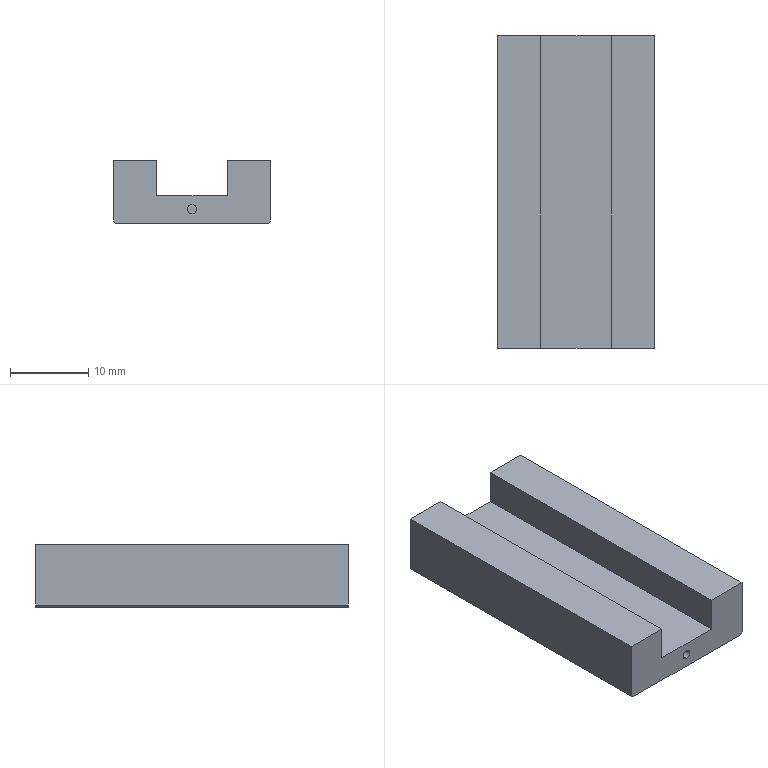Part | SolidWorks | features ICE 3, 3DProfileFeature 1, Chamfer 1, Extrusion 1, HoleWzd 1 | 1 solid | 31 faces | box 20 x 39.9 x 8 mm | volume 4656 mm3 | plane 13 | cylinder 10 | cone 8 | commonest cylinder face diameters 2.5 x8 1.2 x2
STEP:
#1=CARTESIAN_POINT('',(8.75,11.95,1.));
#2=VERTEX_POINT('',#1);
#3=CARTESIAN_POINT('',(6.25,11.95,1.));
#4=VERTEX_POINT('',#3);
#5=CARTESIAN_POINT('',(7.5,11.95,1.));
#6=DIRECTION('',(0.,0.,-1.));
#7=DIRECTION('',(-1.,0.,0.));
#8=AXIS2_PLACEMENT_3D('',#5,#6,#7);
#9=CIRCLE('',#8,1.25);
#10=EDGE_CURVE('',#2,#4,#9,.T.);
#11=ORIENTED_EDGE('',*,*,#10,.F.);
#12=CARTESIAN_POINT('',(8.75,11.95,-4.));
#13=VERTEX_POINT('',#12);
#14=CARTESIAN_POINT('',(8.75,11.95,-4.));
#15=DIRECTION('',(0.,0.,-1.));
#16=VECTOR('',#15,1000.);
#17=LINE('',#14,#16);
#18=EDGE_CURVE('',#2,#13,#17,.T.);
#19=ORIENTED_EDGE('',*,*,#18,.T.);
#20=CARTESIAN_POINT('',(6.25,11.95,-4.));
#21=VERTEX_POINT('',#20);
#22=CARTESIAN_POINT('',(7.5,11.95,-4.));
#23=DIRECTION('',(0.,0.,-1.));
#24=DIRECTION('',(-1.,0.,0.));
#25=AXIS2_PLACEMENT_3D('',#22,#23,#24);
#26=CIRCLE('',#25,1.25);
#27=EDGE_CURVE('',#13,#21,#26,.T.);
#28=ORIENTED_EDGE('',*,*,#27,.T.);
#29=CARTESIAN_POINT('',(6.25,11.95,-4.));
#30=DIRECTION('',(0.,0.,-1.));
#31=VECTOR('',#30,1000.);
#32=LINE('',#29,#31);
#33=EDGE_CURVE('',#4,#21,#32,.T.);
#34=ORIENTED_EDGE('',*,*,#33,.F.);
#35=EDGE_LOOP('',(#11,#19,#28,#34));
#36=FACE_OUTER_BOUND('',#35,.T.);
#37=CARTESIAN_POINT('',(7.5,11.95,-4.));
#38=DIRECTION('',(0.,0.,-1.));
#39=DIRECTION('',(-1.,0.,0.));
#40=AXIS2_PLACEMENT_3D('',#37,#38,#39);
#41=CYLINDRICAL_SURFACE('',#40,1.25);
#42=ADVANCED_FACE('',(#36),#41,.F.);
#43=CARTESIAN_POINT('',(7.5,11.95,1.751));
#44=VERTEX_POINT('',#43);
#45=CARTESIAN_POINT('',(6.25,11.95,1.));
#46=DIRECTION('',(-0.8572,0.,-0.515));
#47=VECTOR('',#46,1000.);
#48=LINE('',#45,#47);
#49=EDGE_CURVE('',#44,#4,#48,.T.);
#50=ORIENTED_EDGE('',*,*,#49,.F.);
#51=CARTESIAN_POINT('',(8.75,11.95,1.));
#52=DIRECTION('',(0.8572,0.,-0.515));
#53=VECTOR('',#52,1000.);
#54=LINE('',#51,#53);
#55=EDGE_CURVE('',#44,#2,#54,.T.);
#56=ORIENTED_EDGE('',*,*,#55,.T.);
#57=ORIENTED_EDGE('',*,*,#10,.T.);
#58=EDGE_LOOP('',(#50,#56,#57));
#59=FACE_OUTER_BOUND('',#58,.T.);
#60=CARTESIAN_POINT('',(7.5,11.95,1.));
#61=DIRECTION('',(0.,0.,-1.));
#62=DIRECTION('',(-1.,0.,0.));
#63=AXIS2_PLACEMENT_3D('',#60,#61,#62);
#64=CONICAL_SURFACE('',#63,1.25,1.03);
#65=ADVANCED_FACE('',(#59),#64,.F.);
#66=CARTESIAN_POINT('',(-6.25,11.95,1.));
#67=VERTEX_POINT('',#66);
#68=CARTESIAN_POINT('',(-8.75,11.95,1.));
#69=VERTEX_POINT('',#68);
#70=CARTESIAN_POINT('',(-7.5,11.95,1.));
#71=DIRECTION('',(0.,0.,-1.));
#72=DIRECTION('',(-1.,0.,0.));
#73=AXIS2_PLACEMENT_3D('',#70,#71,#72);
#74=CIRCLE('',#73,1.25);
#75=EDGE_CURVE('',#67,#69,#74,.T.);
#76=ORIENTED_EDGE('',*,*,#75,.F.);
#77=CARTESIAN_POINT('',(-6.25,11.95,-4.));
#78=VERTEX_POINT('',#77);
#79=CARTESIAN_POINT('',(-6.25,11.95,-4.));
#80=DIRECTION('',(0.,0.,-1.));
#81=VECTOR('',#80,1000.);
#82=LINE('',#79,#81);
#83=EDGE_CURVE('',#67,#78,#82,.T.);
#84=ORIENTED_EDGE('',*,*,#83,.T.);
#85=CARTESIAN_POINT('',(-8.75,11.95,-4.));
#86=VERTEX_POINT('',#85);
#87=CARTESIAN_POINT('',(-7.5,11.95,-4.));
#88=DIRECTION('',(0.,0.,-1.));
#89=DIRECTION('',(-1.,0.,0.));
#90=AXIS2_PLACEMENT_3D('',#87,#88,#89);
#91=CIRCLE('',#90,1.25);
#92=EDGE_CURVE('',#78,#86,#91,.T.);
#93=ORIENTED_EDGE('',*,*,#92,.T.);
#94=CARTESIAN_POINT('',(-8.75,11.95,-4.));
#95=DIRECTION('',(0.,0.,-1.));
#96=VECTOR('',#95,1000.);
#97=LINE('',#94,#96);
#98=EDGE_CURVE('',#69,#86,#97,.T.);
#99=ORIENTED_EDGE('',*,*,#98,.F.);
#100=EDGE_LOOP('',(#76,#84,#93,#99));
#101=FACE_OUTER_BOUND('',#100,.T.);
#102=CARTESIAN_POINT('',(-7.5,11.95,-4.));
#103=DIRECTION('',(0.,0.,-1.));
#104=DIRECTION('',(-1.,0.,0.));
#105=AXIS2_PLACEMENT_3D('',#102,#103,#104);
#106=CYLINDRICAL_SURFACE('',#105,1.25);
#107=ADVANCED_FACE('',(#101),#106,.F.);
#108=CARTESIAN_POINT('',(-7.5,11.95,1.751));
#109=VERTEX_POINT('',#108);
#110=CARTESIAN_POINT('',(-8.75,11.95,1.));
#111=DIRECTION('',(-0.8572,0.,-0.515));
#112=VECTOR('',#111,1000.);
#113=LINE('',#110,#112);
#114=EDGE_CURVE('',#109,#69,#113,.T.);
#115=ORIENTED_EDGE('',*,*,#114,.F.);
#116=CARTESIAN_POINT('',(-6.25,11.95,1.));
#117=DIRECTION('',(0.8572,0.,-0.515));
#118=VECTOR('',#117,1000.);
#119=LINE('',#116,#118);
#120=EDGE_CURVE('',#109,#67,#119,.T.);
#121=ORIENTED_EDGE('',*,*,#120,.T.);
#122=ORIENTED_EDGE('',*,*,#75,.T.);
#123=EDGE_LOOP('',(#115,#121,#122));
#124=FACE_OUTER_BOUND('',#123,.T.);
#125=CARTESIAN_POINT('',(-7.5,11.95,1.));
#126=DIRECTION('',(0.,0.,-1.));
#127=DIRECTION('',(-1.,0.,0.));
#128=AXIS2_PLACEMENT_3D('',#125,#126,#127);
#129=CONICAL_SURFACE('',#128,1.25,1.03);
#130=ADVANCED_FACE('',(#124),#129,.F.);
#131=CARTESIAN_POINT('',(-6.25,27.95,1.));
#132=VERTEX_POINT('',#131);
#133=CARTESIAN_POINT('',(-8.75,27.95,1.));
#134=VERTEX_POINT('',#133);
#135=CARTESIAN_POINT('',(-7.5,27.95,1.));
#136=DIRECTION('',(0.,0.,-1.));
#137=DIRECTION('',(-1.,0.,0.));
#138=AXIS2_PLACEMENT_3D('',#135,#136,#137);
#139=CIRCLE('',#138,1.25);
#140=EDGE_CURVE('',#132,#134,#139,.T.);
#141=ORIENTED_EDGE('',*,*,#140,.F.);
#142=CARTESIAN_POINT('',(-6.25,27.95,-4.));
#143=VERTEX_POINT('',#142);
#144=CARTESIAN_POINT('',(-6.25,27.95,-4.));
#145=DIRECTION('',(0.,0.,-1.));
#146=VECTOR('',#145,1000.);
#147=LINE('',#144,#146);
#148=EDGE_CURVE('',#132,#143,#147,.T.);
#149=ORIENTED_EDGE('',*,*,#148,.T.);
#150=CARTESIAN_POINT('',(-8.75,27.95,-4.));
#151=VERTEX_POINT('',#150);
#152=CARTESIAN_POINT('',(-7.5,27.95,-4.));
#153=DIRECTION('',(0.,0.,-1.));
#154=DIRECTION('',(-1.,0.,0.));
#155=AXIS2_PLACEMENT_3D('',#152,#153,#154);
#156=CIRCLE('',#155,1.25);
#157=EDGE_CURVE('',#143,#151,#156,.T.);
#158=ORIENTED_EDGE('',*,*,#157,.T.);
#159=CARTESIAN_POINT('',(-8.75,27.95,-4.));
#160=DIRECTION('',(0.,0.,-1.));
#161=VECTOR('',#160,1000.);
#162=LINE('',#159,#161);
#163=EDGE_CURVE('',#134,#151,#162,.T.);
#164=ORIENTED_EDGE('',*,*,#163,.F.);
#165=EDGE_LOOP('',(#141,#149,#158,#164));
#166=FACE_OUTER_BOUND('',#165,.T.);
#167=CARTESIAN_POINT('',(-7.5,27.95,-4.));
#168=DIRECTION('',(0.,0.,-1.));
#169=DIRECTION('',(-1.,0.,0.));
#170=AXIS2_PLACEMENT_3D('',#167,#168,#169);
#171=CYLINDRICAL_SURFACE('',#170,1.25);
#172=ADVANCED_FACE('',(#166),#171,.F.);
#173=CARTESIAN_POINT('',(-7.5,27.95,1.751));
#174=VERTEX_POINT('',#173);
#175=CARTESIAN_POINT('',(-8.75,27.95,1.));
#176=DIRECTION('',(-0.8572,0.,-0.515));
#177=VECTOR('',#176,1000.);
#178=LINE('',#175,#177);
#179=EDGE_CURVE('',#174,#134,#178,.T.);
#180=ORIENTED_EDGE('',*,*,#179,.F.);
#181=CARTESIAN_POINT('',(-6.25,27.95,1.));
#182=DIRECTION('',(0.8572,0.,-0.515));
#183=VECTOR('',#182,1000.);
#184=LINE('',#181,#183);
#185=EDGE_CURVE('',#174,#132,#184,.T.);
#186=ORIENTED_EDGE('',*,*,#185,.T.);
#187=ORIENTED_EDGE('',*,*,#140,.T.);
#188=EDGE_LOOP('',(#180,#186,#187));
#189=FACE_OUTER_BOUND('',#188,.T.);
#190=CARTESIAN_POINT('',(-7.5,27.95,1.));
#191=DIRECTION('',(0.,0.,-1.));
#192=DIRECTION('',(-1.,0.,0.));
#193=AXIS2_PLACEMENT_3D('',#190,#191,#192);
#194=CONICAL_SURFACE('',#193,1.25,1.03);
#195=ADVANCED_FACE('',(#189),#194,.F.);
#196=CARTESIAN_POINT('',(8.75,27.95,1.));
#197=VERTEX_POINT('',#196);
#198=CARTESIAN_POINT('',(6.25,27.95,1.));
#199=VERTEX_POINT('',#198);
#200=CARTESIAN_POINT('',(7.5,27.95,1.));
#201=DIRECTION('',(0.,0.,-1.));
#202=DIRECTION('',(-1.,0.,0.));
#203=AXIS2_PLACEMENT_3D('',#200,#201,#202);
#204=CIRCLE('',#203,1.25);
#205=EDGE_CURVE('',#197,#199,#204,.T.);
#206=ORIENTED_EDGE('',*,*,#205,.F.);
#207=CARTESIAN_POINT('',(8.75,27.95,-4.));
#208=VERTEX_POINT('',#207);
#209=CARTESIAN_POINT('',(8.75,27.95,-4.));
#210=DIRECTION('',(0.,0.,-1.));
#211=VECTOR('',#210,1000.);
#212=LINE('',#209,#211);
#213=EDGE_CURVE('',#197,#208,#212,.T.);
#214=ORIENTED_EDGE('',*,*,#213,.T.);
#215=CARTESIAN_POINT('',(6.25,27.95,-4.));
#216=VERTEX_POINT('',#215);
#217=CARTESIAN_POINT('',(7.5,27.95,-4.));
#218=DIRECTION('',(0.,0.,-1.));
#219=DIRECTION('',(-1.,0.,0.));
#220=AXIS2_PLACEMENT_3D('',#217,#218,#219);
#221=CIRCLE('',#220,1.25);
#222=EDGE_CURVE('',#208,#216,#221,.T.);
#223=ORIENTED_EDGE('',*,*,#222,.T.);
#224=CARTESIAN_POINT('',(6.25,27.95,-4.));
#225=DIRECTION('',(0.,0.,-1.));
#226=VECTOR('',#225,1000.);
#227=LINE('',#224,#226);
#228=EDGE_CURVE('',#199,#216,#227,.T.);
#229=ORIENTED_EDGE('',*,*,#228,.F.);
#230=EDGE_LOOP('',(#206,#214,#223,#229));
#231=FACE_OUTER_BOUND('',#230,.T.);
#232=CARTESIAN_POINT('',(7.5,27.95,-4.));
#233=DIRECTION('',(0.,0.,-1.));
#234=DIRECTION('',(-1.,0.,0.));
#235=AXIS2_PLACEMENT_3D('',#232,#233,#234);
#236=CYLINDRICAL_SURFACE('',#235,1.25);
#237=ADVANCED_FACE('',(#231),#236,.F.);
#238=CARTESIAN_POINT('',(7.5,27.95,1.751));
#239=VERTEX_POINT('',#238);
#240=CARTESIAN_POINT('',(6.25,27.95,1.));
#241=DIRECTION('',(-0.8572,0.,-0.515));
#242=VECTOR('',#241,1000.);
#243=LINE('',#240,#242);
#244=EDGE_CURVE('',#239,#199,#243,.T.);
#245=ORIENTED_EDGE('',*,*,#244,.F.);
#246=CARTESIAN_POINT('',(8.75,27.95,1.));
#247=DIRECTION('',(0.8572,0.,-0.515));
#248=VECTOR('',#247,1000.);
#249=LINE('',#246,#248);
#250=EDGE_CURVE('',#239,#197,#249,.T.);
#251=ORIENTED_EDGE('',*,*,#250,.T.);
#252=ORIENTED_EDGE('',*,*,#205,.T.);
#253=EDGE_LOOP('',(#245,#251,#252));
#254=FACE_OUTER_BOUND('',#253,.T.);
#255=CARTESIAN_POINT('',(7.5,27.95,1.));
#256=DIRECTION('',(0.,0.,-1.));
#257=DIRECTION('',(-1.,0.,0.));
#258=AXIS2_PLACEMENT_3D('',#255,#256,#257);
#259=CONICAL_SURFACE('',#258,1.25,1.03);
#260=ADVANCED_FACE('',(#254),#259,.F.);
#261=CARTESIAN_POINT('',(0.,4.5,-1.6));
#262=VERTEX_POINT('',#261);
#263=CARTESIAN_POINT('',(0.,4.5,-2.8));
#264=VERTEX_POINT('',#263);
#265=CARTESIAN_POINT('',(0.,4.5,-2.2));
#266=DIRECTION('',(0.,-1.,0.));
#267=DIRECTION('',(0.,0.,-1.));
#268=AXIS2_PLACEMENT_3D('',#265,#266,#267);
#269=CIRCLE('',#268,0.6);
#270=EDGE_CURVE('',#262,#264,#269,.T.);
#271=ORIENTED_EDGE('',*,*,#270,.F.);
#272=CARTESIAN_POINT('',(0.,0.,-1.6));
#273=VERTEX_POINT('',#272);
#274=CARTESIAN_POINT('',(0.,4.5,-1.6));
#275=DIRECTION('',(0.,-1.,0.));
#276=VECTOR('',#275,1000.);
#277=LINE('',#274,#276);
#278=EDGE_CURVE('',#262,#273,#277,.T.);
#279=ORIENTED_EDGE('',*,*,#278,.T.);
#280=CARTESIAN_POINT('',(0.,0.,-2.8));
#281=VERTEX_POINT('',#280);
#282=CARTESIAN_POINT('',(0.,0.,-2.2));
#283=DIRECTION('',(0.,-1.,0.));
#284=DIRECTION('',(0.,0.,-1.));
#285=AXIS2_PLACEMENT_3D('',#282,#283,#284);
#286=CIRCLE('',#285,0.6);
#287=EDGE_CURVE('',#273,#281,#286,.T.);
#288=ORIENTED_EDGE('',*,*,#287,.T.);
#289=CARTESIAN_POINT('',(0.,4.5,-2.8));
#290=DIRECTION('',(0.,-1.,0.));
#291=VECTOR('',#290,1000.);
#292=LINE('',#289,#291);
#293=EDGE_CURVE('',#264,#281,#292,.T.);
#294=ORIENTED_EDGE('',*,*,#293,.F.);
#295=EDGE_LOOP('',(#271,#279,#288,#294));
#296=FACE_OUTER_BOUND('',#295,.T.);
#297=CARTESIAN_POINT('',(0.,4.5,-2.2));
#298=DIRECTION('',(0.,-1.,0.));
#299=DIRECTION('',(0.,0.,-1.));
#300=AXIS2_PLACEMENT_3D('',#297,#298,#299);
#301=CYLINDRICAL_SURFACE('',#300,0.6);
#302=ADVANCED_FACE('',(#296),#301,.F.);
#303=CARTESIAN_POINT('',(4.5,39.9,4.));
#304=VERTEX_POINT('',#303);
#305=CARTESIAN_POINT('',(10.,39.9,4.));
#306=VERTEX_POINT('',#305);
#307=CARTESIAN_POINT('',(-10.,39.9,4.));
#308=DIRECTION('',(1.,0.,0.));
#309=VECTOR('',#308,1000.);
#310=LINE('',#307,#309);
#311=EDGE_CURVE('',#304,#306,#310,.T.);
#312=ORIENTED_EDGE('',*,*,#311,.F.);
#313=CARTESIAN_POINT('',(4.5,0.,4.));
#314=VERTEX_POINT('',#313);
#315=CARTESIAN_POINT('',(4.5,39.9,4.));
#316=DIRECTION('',(0.,-1.,0.));
#317=VECTOR('',#316,1000.);
#318=LINE('',#315,#317);
#319=EDGE_CURVE('',#304,#314,#318,.T.);
#320=ORIENTED_EDGE('',*,*,#319,.T.);
#321=CARTESIAN_POINT('',(10.,0.,4.));
#322=VERTEX_POINT('',#321);
#323=CARTESIAN_POINT('',(-10.,0.,4.));
#324=DIRECTION('',(1.,0.,0.));
#325=VECTOR('',#324,1000.);
#326=LINE('',#323,#325);
#327=EDGE_CURVE('',#314,#322,#326,.T.);
#328=ORIENTED_EDGE('',*,*,#327,.T.);
#329=CARTESIAN_POINT('',(10.,39.9,4.));
#330=DIRECTION('',(0.,-1.,0.));
#331=VECTOR('',#330,1000.);
#332=LINE('',#329,#331);
#333=EDGE_CURVE('',#306,#322,#332,.T.);
#334=ORIENTED_EDGE('',*,*,#333,.F.);
#335=EDGE_LOOP('',(#312,#320,#328,#334));
#336=FACE_OUTER_BOUND('',#335,.T.);
#337=CARTESIAN_POINT('',(-10.,39.9,4.));
#338=DIRECTION('',(0.,0.,-1.));
#339=DIRECTION('',(-1.,0.,0.));
#340=AXIS2_PLACEMENT_3D('',#337,#338,#339);
#341=PLANE('',#340);
#342=ADVANCED_FACE('',(#336),#341,.F.);
#343=CARTESIAN_POINT('',(10.,0.,-3.7));
#344=VERTEX_POINT('',#343);
#345=CARTESIAN_POINT('',(10.,0.,-4.));
#346=DIRECTION('',(0.,0.,-1.));
#347=VECTOR('',#346,1000.);
#348=LINE('',#345,#347);
#349=EDGE_CURVE('',#322,#344,#348,.T.);
#350=ORIENTED_EDGE('',*,*,#349,.T.);
#351=CARTESIAN_POINT('',(10.,39.9,-3.7));
#352=VERTEX_POINT('',#351);
#353=CARTESIAN_POINT('',(10.,39.9,-3.7));
#354=DIRECTION('',(0.,1.,0.));
#355=VECTOR('',#354,1000.);
#356=LINE('',#353,#355);
#357=EDGE_CURVE('',#344,#352,#356,.T.);
#358=ORIENTED_EDGE('',*,*,#357,.T.);
#359=CARTESIAN_POINT('',(10.,39.9,-4.));
#360=DIRECTION('',(0.,0.,-1.));
#361=VECTOR('',#360,1000.);
#362=LINE('',#359,#361);
#363=EDGE_CURVE('',#306,#352,#362,.T.);
#364=ORIENTED_EDGE('',*,*,#363,.F.);
#365=ORIENTED_EDGE('',*,*,#333,.T.);
#366=EDGE_LOOP('',(#350,#358,#364,#365));
#367=FACE_OUTER_BOUND('',#366,.T.);
#368=CARTESIAN_POINT('',(10.,39.9,-4.));
#369=DIRECTION('',(-1.,0.,0.));
#370=DIRECTION('',(0.,0.,1.));
#371=AXIS2_PLACEMENT_3D('',#368,#369,#370);
#372=PLANE('',#371);
#373=ADVANCED_FACE('',(#367),#372,.F.);
#374=CARTESIAN_POINT('',(7.5,11.95,-4.));
#375=DIRECTION('',(0.,0.,-1.));
#376=DIRECTION('',(-1.,0.,0.));
#377=AXIS2_PLACEMENT_3D('',#374,#375,#376);
#378=CIRCLE('',#377,1.25);
#379=EDGE_CURVE('',#21,#13,#378,.T.);
#380=ORIENTED_EDGE('',*,*,#379,.F.);
#381=ORIENTED_EDGE('',*,*,#27,.F.);
#382=EDGE_LOOP('',(#380,#381));
#383=FACE_BOUND('',#382,.T.);
#384=CARTESIAN_POINT('',(-7.5,11.95,-4.));
#385=DIRECTION('',(0.,0.,-1.));
#386=DIRECTION('',(-1.,0.,0.));
#387=AXIS2_PLACEMENT_3D('',#384,#385,#386);
#388=CIRCLE('',#387,1.25);
#389=EDGE_CURVE('',#86,#78,#388,.T.);
#390=ORIENTED_EDGE('',*,*,#389,.F.);
#391=ORIENTED_EDGE('',*,*,#92,.F.);
#392=EDGE_LOOP('',(#390,#391));
#393=FACE_BOUND('',#392,.T.);
#394=CARTESIAN_POINT('',(-7.5,27.95,-4.));
#395=DIRECTION('',(0.,0.,-1.));
#396=DIRECTION('',(-1.,0.,0.));
#397=AXIS2_PLACEMENT_3D('',#394,#395,#396);
#398=CIRCLE('',#397,1.25);
#399=EDGE_CURVE('',#151,#143,#398,.T.);
#400=ORIENTED_EDGE('',*,*,#399,.F.);
#401=ORIENTED_EDGE('',*,*,#157,.F.);
#402=EDGE_LOOP('',(#400,#401));
#403=FACE_BOUND('',#402,.T.);
#404=CARTESIAN_POINT('',(7.5,27.95,-4.));
#405=DIRECTION('',(0.,0.,-1.));
#406=DIRECTION('',(-1.,0.,0.));
#407=AXIS2_PLACEMENT_3D('',#404,#405,#406);
#408=CIRCLE('',#407,1.25);
#409=EDGE_CURVE('',#216,#208,#408,.T.);
#410=ORIENTED_EDGE('',*,*,#409,.F.);
#411=ORIENTED_EDGE('',*,*,#222,.F.);
#412=EDGE_LOOP('',(#410,#411));
#413=FACE_BOUND('',#412,.T.);
#414=CARTESIAN_POINT('',(9.7,0.,-4.));
#415=VERTEX_POINT('',#414);
#416=CARTESIAN_POINT('',(-9.7,0.,-4.));
#417=VERTEX_POINT('',#416);
#418=CARTESIAN_POINT('',(-10.,0.,-4.));
#419=DIRECTION('',(-1.,0.,0.));
#420=VECTOR('',#419,1000.);
#421=LINE('',#418,#420);
#422=EDGE_CURVE('',#415,#417,#421,.T.);
#423=ORIENTED_EDGE('',*,*,#422,.T.);
#424=CARTESIAN_POINT('',(-9.7,39.9,-4.));
#425=VERTEX_POINT('',#424);
#426=CARTESIAN_POINT('',(-9.7,39.9,-4.));
#427=DIRECTION('',(0.,1.,0.));
#428=VECTOR('',#427,1000.);
#429=LINE('',#426,#428);
#430=EDGE_CURVE('',#417,#425,#429,.T.);
#431=ORIENTED_EDGE('',*,*,#430,.T.);
#432=CARTESIAN_POINT('',(9.7,39.9,-4.));
#433=VERTEX_POINT('',#432);
#434=CARTESIAN_POINT('',(-10.,39.9,-4.));
#435=DIRECTION('',(-1.,0.,0.));
#436=VECTOR('',#435,1000.);
#437=LINE('',#434,#436);
#438=EDGE_CURVE('',#433,#425,#437,.T.);
#439=ORIENTED_EDGE('',*,*,#438,.F.);
#440=CARTESIAN_POINT('',(9.7,39.9,-4.));
#441=DIRECTION('',(0.,-1.,0.));
#442=VECTOR('',#441,1000.);
#443=LINE('',#440,#442);
#444=EDGE_CURVE('',#433,#415,#443,.T.);
#445=ORIENTED_EDGE('',*,*,#444,.T.);
#446=EDGE_LOOP('',(#423,#431,#439,#445));
#447=FACE_OUTER_BOUND('',#446,.T.);
#448=CARTESIAN_POINT('',(-10.,39.9,-4.));
#449=DIRECTION('',(0.,0.,1.));
#450=DIRECTION('',(1.,0.,0.));
#451=AXIS2_PLACEMENT_3D('',#448,#449,#450);
#452=PLANE('',#451);
#453=ADVANCED_FACE('',(#383,#393,#403,#413,#447),#452,.F.);
#454=CARTESIAN_POINT('',(-10.,39.9,-3.7));
#455=VERTEX_POINT('',#454);
#456=CARTESIAN_POINT('',(-10.,39.9,4.));
#457=VERTEX_POINT('',#456);
#458=CARTESIAN_POINT('',(-10.,39.9,-4.));
#459=DIRECTION('',(0.,0.,1.));
#460=VECTOR('',#459,1000.);
#461=LINE('',#458,#460);
#462=EDGE_CURVE('',#455,#457,#461,.T.);
#463=ORIENTED_EDGE('',*,*,#462,.F.);
#464=CARTESIAN_POINT('',(-10.,0.,-3.7));
#465=VERTEX_POINT('',#464);
#466=CARTESIAN_POINT('',(-10.,39.9,-3.7));
#467=DIRECTION('',(0.,-1.,0.));
#468=VECTOR('',#467,1000.);
#469=LINE('',#466,#468);
#470=EDGE_CURVE('',#455,#465,#469,.T.);
#471=ORIENTED_EDGE('',*,*,#470,.T.);
#472=CARTESIAN_POINT('',(-10.,0.,4.));
#473=VERTEX_POINT('',#472);
#474=CARTESIAN_POINT('',(-10.,0.,-4.));
#475=DIRECTION('',(0.,0.,1.));
#476=VECTOR('',#475,1000.);
#477=LINE('',#474,#476);
#478=EDGE_CURVE('',#465,#473,#477,.T.);
#479=ORIENTED_EDGE('',*,*,#478,.T.);
#480=CARTESIAN_POINT('',(-10.,39.9,4.));
#481=DIRECTION('',(0.,-1.,0.));
#482=VECTOR('',#481,1000.);
#483=LINE('',#480,#482);
#484=EDGE_CURVE('',#457,#473,#483,.T.);
#485=ORIENTED_EDGE('',*,*,#484,.F.);
#486=EDGE_LOOP('',(#463,#471,#479,#485));
#487=FACE_OUTER_BOUND('',#486,.T.);
#488=CARTESIAN_POINT('',(-10.,39.9,-4.));
#489=DIRECTION('',(1.,0.,0.));
#490=DIRECTION('',(0.,0.,-1.));
#491=AXIS2_PLACEMENT_3D('',#488,#489,#490);
#492=PLANE('',#491);
#493=ADVANCED_FACE('',(#487),#492,.F.);
#494=CARTESIAN_POINT('',(-4.5,0.,4.));
#495=VERTEX_POINT('',#494);
#496=CARTESIAN_POINT('',(-10.,0.,4.));
#497=DIRECTION('',(1.,0.,0.));
#498=VECTOR('',#497,1000.);
#499=LINE('',#496,#498);
#500=EDGE_CURVE('',#473,#495,#499,.T.);
#501=ORIENTED_EDGE('',*,*,#500,.T.);
#502=CARTESIAN_POINT('',(-4.5,39.9,4.));
#503=VERTEX_POINT('',#502);
#504=CARTESIAN_POINT('',(-4.5,39.9,4.));
#505=DIRECTION('',(0.,1.,0.));
#506=VECTOR('',#505,1000.);
#507=LINE('',#504,#506);
#508=EDGE_CURVE('',#495,#503,#507,.T.);
#509=ORIENTED_EDGE('',*,*,#508,.T.);
#510=CARTESIAN_POINT('',(-10.,39.9,4.));
#511=DIRECTION('',(1.,0.,0.));
#512=VECTOR('',#511,1000.);
#513=LINE('',#510,#512);
#514=EDGE_CURVE('',#457,#503,#513,.T.);
#515=ORIENTED_EDGE('',*,*,#514,.F.);
#516=ORIENTED_EDGE('',*,*,#484,.T.);
#517=EDGE_LOOP('',(#501,#509,#515,#516));
#518=FACE_OUTER_BOUND('',#517,.T.);
#519=CARTESIAN_POINT('',(-10.,39.9,4.));
#520=DIRECTION('',(0.,0.,-1.));
#521=DIRECTION('',(-1.,0.,0.));
#522=AXIS2_PLACEMENT_3D('',#519,#520,#521);
#523=PLANE('',#522);
#524=ADVANCED_FACE('',(#518),#523,.F.);
#525=ORIENTED_EDGE('',*,*,#438,.T.);
#526=CARTESIAN_POINT('',(-6.85,39.9,-6.85));
#527=DIRECTION('',(-0.7071,0.,0.7071));
#528=VECTOR('',#527,1000.);
#529=LINE('',#526,#528);
#530=EDGE_CURVE('',#425,#455,#529,.T.);
#531=ORIENTED_EDGE('',*,*,#530,.T.);
#532=ORIENTED_EDGE('',*,*,#462,.T.);
#533=ORIENTED_EDGE('',*,*,#514,.T.);
#534=CARTESIAN_POINT('',(-4.5,39.9,-0.5));
#535=VERTEX_POINT('',#534);
#536=CARTESIAN_POINT('',(-4.5,39.9,8.5));
#537=DIRECTION('',(0.,0.,1.));
#538=VECTOR('',#537,1000.);
#539=LINE('',#536,#538);
#540=EDGE_CURVE('',#535,#503,#539,.T.);
#541=ORIENTED_EDGE('',*,*,#540,.F.);
#542=CARTESIAN_POINT('',(4.5,39.9,-0.5));
#543=VERTEX_POINT('',#542);
#544=CARTESIAN_POINT('',(-4.5,39.9,-0.5));
#545=DIRECTION('',(-1.,0.,0.));
#546=VECTOR('',#545,1000.);
#547=LINE('',#544,#546);
#548=EDGE_CURVE('',#543,#535,#547,.T.);
#549=ORIENTED_EDGE('',*,*,#548,.F.);
#550=CARTESIAN_POINT('',(4.5,39.9,8.5));
#551=DIRECTION('',(0.,0.,-1.));
#552=VECTOR('',#551,1000.);
#553=LINE('',#550,#552);
#554=EDGE_CURVE('',#304,#543,#553,.T.);
#555=ORIENTED_EDGE('',*,*,#554,.F.);
#556=ORIENTED_EDGE('',*,*,#311,.T.);
#557=ORIENTED_EDGE('',*,*,#363,.T.);
#558=CARTESIAN_POINT('',(6.85,39.9,-6.85));
#559=DIRECTION('',(-0.7071,0.,-0.7071));
#560=VECTOR('',#559,1000.);
#561=LINE('',#558,#560);
#562=EDGE_CURVE('',#352,#433,#561,.T.);
#563=ORIENTED_EDGE('',*,*,#562,.T.);
#564=EDGE_LOOP('',(#525,#531,#532,#533,#541,#549,#555,#556,#557,#563));
#565=FACE_OUTER_BOUND('',#564,.T.);
#566=CARTESIAN_POINT('',(0.,39.9,0.));
#567=DIRECTION('',(0.,1.,0.));
#568=DIRECTION('',(0.,0.,1.));
#569=AXIS2_PLACEMENT_3D('',#566,#567,#568);
#570=PLANE('',#569);
#571=ADVANCED_FACE('',(#565),#570,.T.);
#572=CARTESIAN_POINT('',(0.,0.,-2.2));
#573=DIRECTION('',(0.,-1.,0.));
#574=DIRECTION('',(0.,0.,-1.));
#575=AXIS2_PLACEMENT_3D('',#572,#573,#574);
#576=CIRCLE('',#575,0.6);
#577=EDGE_CURVE('',#281,#273,#576,.T.);
#578=ORIENTED_EDGE('',*,*,#577,.F.);
#579=ORIENTED_EDGE('',*,*,#287,.F.);
#580=EDGE_LOOP('',(#578,#579));
#581=FACE_BOUND('',#580,.T.);
#582=ORIENTED_EDGE('',*,*,#478,.F.);
#583=CARTESIAN_POINT('',(-10.,0.,-3.7));
#584=DIRECTION('',(0.7071,0.,-0.7071));
#585=VECTOR('',#584,1000.);
#586=LINE('',#583,#585);
#587=EDGE_CURVE('',#465,#417,#586,.T.);
#588=ORIENTED_EDGE('',*,*,#587,.T.);
#589=ORIENTED_EDGE('',*,*,#422,.F.);
#590=CARTESIAN_POINT('',(9.7,0.,-4.));
#591=DIRECTION('',(0.7071,0.,0.7071));
#592=VECTOR('',#591,1000.);
#593=LINE('',#590,#592);
#594=EDGE_CURVE('',#415,#344,#593,.T.);
#595=ORIENTED_EDGE('',*,*,#594,.T.);
#596=ORIENTED_EDGE('',*,*,#349,.F.);
#597=ORIENTED_EDGE('',*,*,#327,.F.);
#598=CARTESIAN_POINT('',(4.5,0.,-0.5));
#599=VERTEX_POINT('',#598);
#600=CARTESIAN_POINT('',(4.5,0.,0.));
#601=DIRECTION('',(0.,0.,-1.));
#602=VECTOR('',#601,1000.);
#603=LINE('',#600,#602);
#604=EDGE_CURVE('',#314,#599,#603,.T.);
#605=ORIENTED_EDGE('',*,*,#604,.T.);
#606=CARTESIAN_POINT('',(-4.5,0.,-0.5));
#607=VERTEX_POINT('',#606);
#608=CARTESIAN_POINT('',(-4.5,0.,-0.5));
#609=DIRECTION('',(-1.,0.,0.));
#610=VECTOR('',#609,1000.);
#611=LINE('',#608,#610);
#612=EDGE_CURVE('',#599,#607,#611,.T.);
#613=ORIENTED_EDGE('',*,*,#612,.T.);
#614=CARTESIAN_POINT('',(-4.5,0.,8.5));
#615=DIRECTION('',(0.,0.,1.));
#616=VECTOR('',#615,1000.);
#617=LINE('',#614,#616);
#618=EDGE_CURVE('',#607,#495,#617,.T.);
#619=ORIENTED_EDGE('',*,*,#618,.T.);
#620=ORIENTED_EDGE('',*,*,#500,.F.);
#621=EDGE_LOOP('',(#582,#588,#589,#595,#596,#597,#605,#613,#619,#620));
#622=FACE_OUTER_BOUND('',#621,.T.);
#623=CARTESIAN_POINT('',(0.,0.,0.));
#624=DIRECTION('',(0.,1.,0.));
#625=DIRECTION('',(0.,0.,1.));
#626=AXIS2_PLACEMENT_3D('',#623,#624,#625);
#627=PLANE('',#626);
#628=ADVANCED_FACE('',(#581,#622),#627,.F.);
#629=ORIENTED_EDGE('',*,*,#554,.T.);
#630=CARTESIAN_POINT('',(4.5,0.,-0.5));
#631=DIRECTION('',(0.,1.,0.));
#632=VECTOR('',#631,1000.);
#633=LINE('',#630,#632);
#634=EDGE_CURVE('',#599,#543,#633,.T.);
#635=ORIENTED_EDGE('',*,*,#634,.F.);
#636=ORIENTED_EDGE('',*,*,#604,.F.);
#637=ORIENTED_EDGE('',*,*,#319,.F.);
#638=EDGE_LOOP('',(#629,#635,#636,#637));
#639=FACE_OUTER_BOUND('',#638,.T.);
#640=CARTESIAN_POINT('',(4.5,0.,8.5));
#641=DIRECTION('',(1.,0.,0.));
#642=DIRECTION('',(0.,0.,-1.));
#643=AXIS2_PLACEMENT_3D('',#640,#641,#642);
#644=PLANE('',#643);
#645=ADVANCED_FACE('',(#639),#644,.F.);
#646=ORIENTED_EDGE('',*,*,#618,.F.);
#647=CARTESIAN_POINT('',(-4.5,0.,-0.5));
#648=DIRECTION('',(0.,1.,0.));
#649=VECTOR('',#648,1000.);
#650=LINE('',#647,#649);
#651=EDGE_CURVE('',#607,#535,#650,.T.);
#652=ORIENTED_EDGE('',*,*,#651,.T.);
#653=ORIENTED_EDGE('',*,*,#540,.T.);
#654=ORIENTED_EDGE('',*,*,#508,.F.);
#655=EDGE_LOOP('',(#646,#652,#653,#654));
#656=FACE_OUTER_BOUND('',#655,.T.);
#657=CARTESIAN_POINT('',(-4.5,0.,8.5));
#658=DIRECTION('',(-1.,0.,0.));
#659=DIRECTION('',(0.,0.,1.));
#660=AXIS2_PLACEMENT_3D('',#657,#658,#659);
#661=PLANE('',#660);
#662=ADVANCED_FACE('',(#656),#661,.F.);
#663=ORIENTED_EDGE('',*,*,#548,.T.);
#664=ORIENTED_EDGE('',*,*,#651,.F.);
#665=ORIENTED_EDGE('',*,*,#612,.F.);
#666=ORIENTED_EDGE('',*,*,#634,.T.);
#667=EDGE_LOOP('',(#663,#664,#665,#666));
#668=FACE_OUTER_BOUND('',#667,.T.);
#669=CARTESIAN_POINT('',(-4.5,0.,-0.5));
#670=DIRECTION('',(0.,0.,-1.));
#671=DIRECTION('',(-1.,0.,0.));
#672=AXIS2_PLACEMENT_3D('',#669,#670,#671);
#673=PLANE('',#672);
#674=ADVANCED_FACE('',(#668),#673,.F.);
#675=ORIENTED_EDGE('',*,*,#530,.F.);
#676=ORIENTED_EDGE('',*,*,#430,.F.);
#677=ORIENTED_EDGE('',*,*,#587,.F.);
#678=ORIENTED_EDGE('',*,*,#470,.F.);
#679=EDGE_LOOP('',(#675,#676,#677,#678));
#680=FACE_OUTER_BOUND('',#679,.T.);
#681=CARTESIAN_POINT('',(-10.,39.9,-3.7));
#682=DIRECTION('',(0.7071,0.,0.7071));
#683=DIRECTION('',(0.,-1.,0.));
#684=AXIS2_PLACEMENT_3D('',#681,#682,#683);
#685=PLANE('',#684);
#686=ADVANCED_FACE('',(#680),#685,.F.);
#687=ORIENTED_EDGE('',*,*,#562,.F.);
#688=ORIENTED_EDGE('',*,*,#357,.F.);
#689=ORIENTED_EDGE('',*,*,#594,.F.);
#690=ORIENTED_EDGE('',*,*,#444,.F.);
#691=EDGE_LOOP('',(#687,#688,#689,#690));
#692=FACE_OUTER_BOUND('',#691,.T.);
#693=CARTESIAN_POINT('',(9.7,39.9,-4.));
#694=DIRECTION('',(-0.7071,0.,0.7071));
#695=DIRECTION('',(0.,-1.,0.));
#696=AXIS2_PLACEMENT_3D('',#693,#694,#695);
#697=PLANE('',#696);
#698=ADVANCED_FACE('',(#692),#697,.F.);
#699=ORIENTED_EDGE('',*,*,#278,.F.);
#700=CARTESIAN_POINT('',(0.,4.5,-2.2));
#701=DIRECTION('',(0.,-1.,0.));
#702=DIRECTION('',(0.,0.,-1.));
#703=AXIS2_PLACEMENT_3D('',#700,#701,#702);
#704=CIRCLE('',#703,0.6);
#705=EDGE_CURVE('',#264,#262,#704,.T.);
#706=ORIENTED_EDGE('',*,*,#705,.F.);
#707=ORIENTED_EDGE('',*,*,#293,.T.);
#708=ORIENTED_EDGE('',*,*,#577,.T.);
#709=EDGE_LOOP('',(#699,#706,#707,#708));
#710=FACE_OUTER_BOUND('',#709,.T.);
#711=CARTESIAN_POINT('',(0.,4.5,-2.2));
#712=DIRECTION('',(0.,-1.,0.));
#713=DIRECTION('',(0.,0.,-1.));
#714=AXIS2_PLACEMENT_3D('',#711,#712,#713);
#715=CYLINDRICAL_SURFACE('',#714,0.6);
#716=ADVANCED_FACE('',(#710),#715,.F.);
#717=ORIENTED_EDGE('',*,*,#705,.T.);
#718=ORIENTED_EDGE('',*,*,#270,.T.);
#719=EDGE_LOOP('',(#717,#718));
#720=FACE_OUTER_BOUND('',#719,.T.);
#721=CARTESIAN_POINT('',(0.,4.5,-2.2));
#722=DIRECTION('',(0.,-1.,0.));
#723=DIRECTION('',(0.,0.,-1.));
#724=AXIS2_PLACEMENT_3D('',#721,#722,#723);
#725=PLANE('',#724);
#726=ADVANCED_FACE('',(#720),#725,.T.);
#727=ORIENTED_EDGE('',*,*,#250,.F.);
#728=ORIENTED_EDGE('',*,*,#244,.T.);
#729=CARTESIAN_POINT('',(7.5,27.95,1.));
#730=DIRECTION('',(0.,0.,-1.));
#731=DIRECTION('',(-1.,0.,0.));
#732=AXIS2_PLACEMENT_3D('',#729,#730,#731);
#733=CIRCLE('',#732,1.25);
#734=EDGE_CURVE('',#199,#197,#733,.T.);
#735=ORIENTED_EDGE('',*,*,#734,.T.);
#736=EDGE_LOOP('',(#727,#728,#735));
#737=FACE_OUTER_BOUND('',#736,.T.);
#738=CARTESIAN_POINT('',(7.5,27.95,1.));
#739=DIRECTION('',(0.,0.,-1.));
#740=DIRECTION('',(-1.,0.,0.));
#741=AXIS2_PLACEMENT_3D('',#738,#739,#740);
#742=CONICAL_SURFACE('',#741,1.25,1.03);
#743=ADVANCED_FACE('',(#737),#742,.F.);
#744=ORIENTED_EDGE('',*,*,#213,.F.);
#745=ORIENTED_EDGE('',*,*,#734,.F.);
#746=ORIENTED_EDGE('',*,*,#228,.T.);
#747=ORIENTED_EDGE('',*,*,#409,.T.);
#748=EDGE_LOOP('',(#744,#745,#746,#747));
#749=FACE_OUTER_BOUND('',#748,.T.);
#750=CARTESIAN_POINT('',(7.5,27.95,-4.));
#751=DIRECTION('',(0.,0.,-1.));
#752=DIRECTION('',(-1.,0.,0.));
#753=AXIS2_PLACEMENT_3D('',#750,#751,#752);
#754=CYLINDRICAL_SURFACE('',#753,1.25);
#755=ADVANCED_FACE('',(#749),#754,.F.);
#756=ORIENTED_EDGE('',*,*,#185,.F.);
#757=ORIENTED_EDGE('',*,*,#179,.T.);
#758=CARTESIAN_POINT('',(-7.5,27.95,1.));
#759=DIRECTION('',(0.,0.,-1.));
#760=DIRECTION('',(-1.,0.,0.));
#761=AXIS2_PLACEMENT_3D('',#758,#759,#760);
#762=CIRCLE('',#761,1.25);
#763=EDGE_CURVE('',#134,#132,#762,.T.);
#764=ORIENTED_EDGE('',*,*,#763,.T.);
#765=EDGE_LOOP('',(#756,#757,#764));
#766=FACE_OUTER_BOUND('',#765,.T.);
#767=CARTESIAN_POINT('',(-7.5,27.95,1.));
#768=DIRECTION('',(0.,0.,-1.));
#769=DIRECTION('',(-1.,0.,0.));
#770=AXIS2_PLACEMENT_3D('',#767,#768,#769);
#771=CONICAL_SURFACE('',#770,1.25,1.03);
#772=ADVANCED_FACE('',(#766),#771,.F.);
#773=ORIENTED_EDGE('',*,*,#148,.F.);
#774=ORIENTED_EDGE('',*,*,#763,.F.);
#775=ORIENTED_EDGE('',*,*,#163,.T.);
#776=ORIENTED_EDGE('',*,*,#399,.T.);
#777=EDGE_LOOP('',(#773,#774,#775,#776));
#778=FACE_OUTER_BOUND('',#777,.T.);
#779=CARTESIAN_POINT('',(-7.5,27.95,-4.));
#780=DIRECTION('',(0.,0.,-1.));
#781=DIRECTION('',(-1.,0.,0.));
#782=AXIS2_PLACEMENT_3D('',#779,#780,#781);
#783=CYLINDRICAL_SURFACE('',#782,1.25);
#784=ADVANCED_FACE('',(#778),#783,.F.);
#785=ORIENTED_EDGE('',*,*,#120,.F.);
#786=ORIENTED_EDGE('',*,*,#114,.T.);
#787=CARTESIAN_POINT('',(-7.5,11.95,1.));
#788=DIRECTION('',(0.,0.,-1.));
#789=DIRECTION('',(-1.,0.,0.));
#790=AXIS2_PLACEMENT_3D('',#787,#788,#789);
#791=CIRCLE('',#790,1.25);
#792=EDGE_CURVE('',#69,#67,#791,.T.);
#793=ORIENTED_EDGE('',*,*,#792,.T.);
#794=EDGE_LOOP('',(#785,#786,#793));
#795=FACE_OUTER_BOUND('',#794,.T.);
#796=CARTESIAN_POINT('',(-7.5,11.95,1.));
#797=DIRECTION('',(0.,0.,-1.));
#798=DIRECTION('',(-1.,0.,0.));
#799=AXIS2_PLACEMENT_3D('',#796,#797,#798);
#800=CONICAL_SURFACE('',#799,1.25,1.03);
#801=ADVANCED_FACE('',(#795),#800,.F.);
#802=ORIENTED_EDGE('',*,*,#83,.F.);
#803=ORIENTED_EDGE('',*,*,#792,.F.);
#804=ORIENTED_EDGE('',*,*,#98,.T.);
#805=ORIENTED_EDGE('',*,*,#389,.T.);
#806=EDGE_LOOP('',(#802,#803,#804,#805));
#807=FACE_OUTER_BOUND('',#806,.T.);
#808=CARTESIAN_POINT('',(-7.5,11.95,-4.));
#809=DIRECTION('',(0.,0.,-1.));
#810=DIRECTION('',(-1.,0.,0.));
#811=AXIS2_PLACEMENT_3D('',#808,#809,#810);
#812=CYLINDRICAL_SURFACE('',#811,1.25);
#813=ADVANCED_FACE('',(#807),#812,.F.);
#814=ORIENTED_EDGE('',*,*,#55,.F.);
#815=ORIENTED_EDGE('',*,*,#49,.T.);
#816=CARTESIAN_POINT('',(7.5,11.95,1.));
#817=DIRECTION('',(0.,0.,-1.));
#818=DIRECTION('',(-1.,0.,0.));
#819=AXIS2_PLACEMENT_3D('',#816,#817,#818);
#820=CIRCLE('',#819,1.25);
#821=EDGE_CURVE('',#4,#2,#820,.T.);
#822=ORIENTED_EDGE('',*,*,#821,.T.);
#823=EDGE_LOOP('',(#814,#815,#822));
#824=FACE_OUTER_BOUND('',#823,.T.);
#825=CARTESIAN_POINT('',(7.5,11.95,1.));
#826=DIRECTION('',(0.,0.,-1.));
#827=DIRECTION('',(-1.,0.,0.));
#828=AXIS2_PLACEMENT_3D('',#825,#826,#827);
#829=CONICAL_SURFACE('',#828,1.25,1.03);
#830=ADVANCED_FACE('',(#824),#829,.F.);
#831=ORIENTED_EDGE('',*,*,#18,.F.);
#832=ORIENTED_EDGE('',*,*,#821,.F.);
#833=ORIENTED_EDGE('',*,*,#33,.T.);
#834=ORIENTED_EDGE('',*,*,#379,.T.);
#835=EDGE_LOOP('',(#831,#832,#833,#834));
#836=FACE_OUTER_BOUND('',#835,.T.);
#837=CARTESIAN_POINT('',(7.5,11.95,-4.));
#838=DIRECTION('',(0.,0.,-1.));
#839=DIRECTION('',(-1.,0.,0.));
#840=AXIS2_PLACEMENT_3D('',#837,#838,#839);
#841=CYLINDRICAL_SURFACE('',#840,1.25);
#842=ADVANCED_FACE('',(#836),#841,.F.);
#843=CLOSED_SHELL('',(#42,#65,#107,#130,#172,#195,#237,#260,#302,#342,#373,#453,#493,#524,#571,#628,#645,#662,#674,#686,#698,#716,#726,#743,#755,#772,#784,#801,#813,#830,#842));
#844=MANIFOLD_SOLID_BREP('',#843);
#845=CARTESIAN_POINT('',(0.,0.,0.));
#846=DIRECTION('',(0.,0.,1.));
#847=DIRECTION('',(1.,0.,0.));
#848=AXIS2_PLACEMENT_3D('',#845,#846,#847);
#849=(LENGTH_UNIT()NAMED_UNIT(*)SI_UNIT(.MILLI.,.METRE.));
#850=UNCERTAINTY_MEASURE_WITH_UNIT(LENGTH_MEASURE(0.00001),#849,'','');
#851=(NAMED_UNIT(*)PLANE_ANGLE_UNIT()SI_UNIT($,.RADIAN.));
#852=(NAMED_UNIT(*)SI_UNIT($,.STERADIAN.)SOLID_ANGLE_UNIT());
#853=(GEOMETRIC_REPRESENTATION_CONTEXT(3)GLOBAL_UNCERTAINTY_ASSIGNED_CONTEXT((#850))GLOBAL_UNIT_ASSIGNED_CONTEXT((#849,#851,#852))REPRESENTATION_CONTEXT('',''));
#854=ADVANCED_BREP_SHAPE_REPRESENTATION('',(#844,#848),#853);